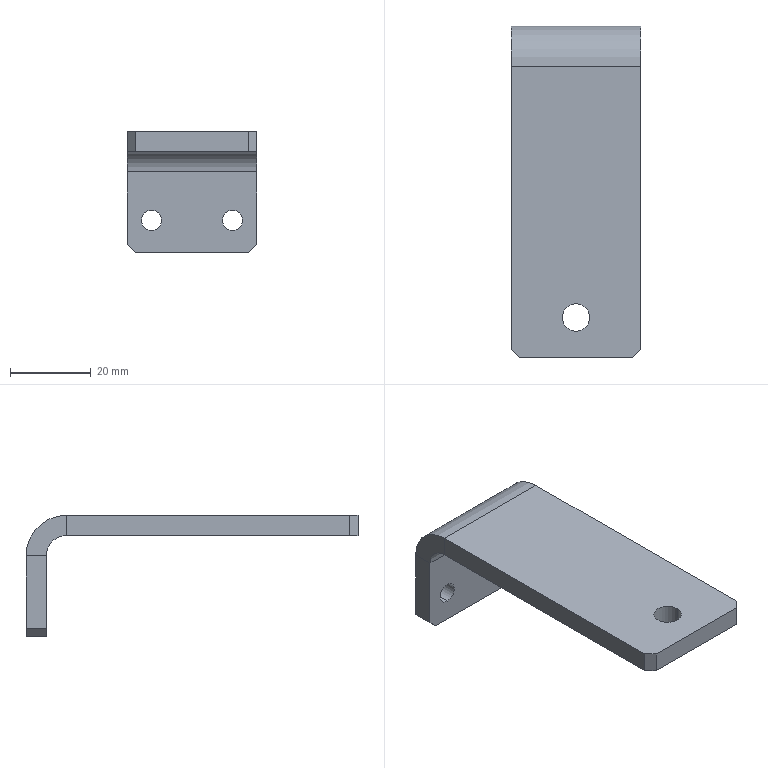Part | SolidWorks | features HoleWzd 2, Chamfer 1, EdgeFlange 1, FlatPattern 1, SMBaseFlange 1, SheetMetal 1 | 1 solid | 24 faces | box 32 x 82 x 30 mm | volume 16187 mm3 | plane 16 | cylinder 8 | commonest cylinder face diameters 5 x4 6.8 x2 10 x1 20 x1
STEP:
#1=CARTESIAN_POINT('',(-5.502,-25.632,-5.));
#2=VERTEX_POINT('',#1);
#3=CARTESIAN_POINT('',(1.298,-25.632,-5.));
#4=VERTEX_POINT('',#3);
#5=CARTESIAN_POINT('',(-2.102,-25.632,-5.));
#6=DIRECTION('',(0.,0.,1.));
#7=DIRECTION('',(1.,0.,0.));
#8=AXIS2_PLACEMENT_3D('',#5,#6,#7);
#9=CIRCLE('',#8,3.4);
#10=EDGE_CURVE('',#2,#4,#9,.T.);
#11=ORIENTED_EDGE('',*,*,#10,.F.);
#12=CARTESIAN_POINT('',(-5.502,-25.632,0.));
#13=VERTEX_POINT('',#12);
#14=CARTESIAN_POINT('',(-5.502,-25.632,0.));
#15=DIRECTION('',(0.,0.,1.));
#16=VECTOR('',#15,1000.);
#17=LINE('',#14,#16);
#18=EDGE_CURVE('',#2,#13,#17,.T.);
#19=ORIENTED_EDGE('',*,*,#18,.T.);
#20=CARTESIAN_POINT('',(1.298,-25.632,0.));
#21=VERTEX_POINT('',#20);
#22=CARTESIAN_POINT('',(-2.102,-25.632,0.));
#23=DIRECTION('',(0.,0.,1.));
#24=DIRECTION('',(1.,0.,0.));
#25=AXIS2_PLACEMENT_3D('',#22,#23,#24);
#26=CIRCLE('',#25,3.4);
#27=EDGE_CURVE('',#13,#21,#26,.T.);
#28=ORIENTED_EDGE('',*,*,#27,.T.);
#29=CARTESIAN_POINT('',(1.298,-25.632,0.));
#30=DIRECTION('',(0.,0.,1.));
#31=VECTOR('',#30,1000.);
#32=LINE('',#29,#31);
#33=EDGE_CURVE('',#4,#21,#32,.T.);
#34=ORIENTED_EDGE('',*,*,#33,.F.);
#35=EDGE_LOOP('',(#11,#19,#28,#34));
#36=FACE_OUTER_BOUND('',#35,.T.);
#37=CARTESIAN_POINT('',(-2.102,-25.632,0.));
#38=DIRECTION('',(0.,0.,1.));
#39=DIRECTION('',(1.,0.,0.));
#40=AXIS2_PLACEMENT_3D('',#37,#38,#39);
#41=CYLINDRICAL_SURFACE('',#40,3.4);
#42=ADVANCED_FACE('',(#36),#41,.F.);
#43=CARTESIAN_POINT('',(-12.102,41.368,-24.5));
#44=VERTEX_POINT('',#43);
#45=CARTESIAN_POINT('',(-12.102,41.368,-19.5));
#46=VERTEX_POINT('',#45);
#47=CARTESIAN_POINT('',(-12.102,41.368,-22.));
#48=DIRECTION('',(0.,1.,0.));
#49=DIRECTION('',(0.,0.,1.));
#50=AXIS2_PLACEMENT_3D('',#47,#48,#49);
#51=CIRCLE('',#50,2.5);
#52=EDGE_CURVE('',#44,#46,#51,.T.);
#53=ORIENTED_EDGE('',*,*,#52,.F.);
#54=CARTESIAN_POINT('',(-12.102,46.368,-24.5));
#55=VERTEX_POINT('',#54);
#56=CARTESIAN_POINT('',(-12.102,46.368,-24.5));
#57=DIRECTION('',(0.,1.,0.));
#58=VECTOR('',#57,1000.);
#59=LINE('',#56,#58);
#60=EDGE_CURVE('',#44,#55,#59,.T.);
#61=ORIENTED_EDGE('',*,*,#60,.T.);
#62=CARTESIAN_POINT('',(-12.102,46.368,-19.5));
#63=VERTEX_POINT('',#62);
#64=CARTESIAN_POINT('',(-12.102,46.368,-22.));
#65=DIRECTION('',(0.,1.,0.));
#66=DIRECTION('',(0.,0.,1.));
#67=AXIS2_PLACEMENT_3D('',#64,#65,#66);
#68=CIRCLE('',#67,2.5);
#69=EDGE_CURVE('',#55,#63,#68,.T.);
#70=ORIENTED_EDGE('',*,*,#69,.T.);
#71=CARTESIAN_POINT('',(-12.102,46.368,-19.5));
#72=DIRECTION('',(0.,1.,0.));
#73=VECTOR('',#72,1000.);
#74=LINE('',#71,#73);
#75=EDGE_CURVE('',#46,#63,#74,.T.);
#76=ORIENTED_EDGE('',*,*,#75,.F.);
#77=EDGE_LOOP('',(#53,#61,#70,#76));
#78=FACE_OUTER_BOUND('',#77,.T.);
#79=CARTESIAN_POINT('',(-12.102,46.368,-22.));
#80=DIRECTION('',(0.,1.,0.));
#81=DIRECTION('',(0.,0.,1.));
#82=AXIS2_PLACEMENT_3D('',#79,#80,#81);
#83=CYLINDRICAL_SURFACE('',#82,2.5);
#84=ADVANCED_FACE('',(#78),#83,.F.);
#85=CARTESIAN_POINT('',(7.898,41.368,-24.5));
#86=VERTEX_POINT('',#85);
#87=CARTESIAN_POINT('',(7.898,41.368,-19.5));
#88=VERTEX_POINT('',#87);
#89=CARTESIAN_POINT('',(7.898,41.368,-22.));
#90=DIRECTION('',(0.,1.,0.));
#91=DIRECTION('',(0.,0.,1.));
#92=AXIS2_PLACEMENT_3D('',#89,#90,#91);
#93=CIRCLE('',#92,2.5);
#94=EDGE_CURVE('',#86,#88,#93,.T.);
#95=ORIENTED_EDGE('',*,*,#94,.F.);
#96=CARTESIAN_POINT('',(7.898,46.368,-24.5));
#97=VERTEX_POINT('',#96);
#98=CARTESIAN_POINT('',(7.898,46.368,-24.5));
#99=DIRECTION('',(0.,1.,0.));
#100=VECTOR('',#99,1000.);
#101=LINE('',#98,#100);
#102=EDGE_CURVE('',#86,#97,#101,.T.);
#103=ORIENTED_EDGE('',*,*,#102,.T.);
#104=CARTESIAN_POINT('',(7.898,46.368,-19.5));
#105=VERTEX_POINT('',#104);
#106=CARTESIAN_POINT('',(7.898,46.368,-22.));
#107=DIRECTION('',(0.,1.,0.));
#108=DIRECTION('',(0.,0.,1.));
#109=AXIS2_PLACEMENT_3D('',#106,#107,#108);
#110=CIRCLE('',#109,2.5);
#111=EDGE_CURVE('',#97,#105,#110,.T.);
#112=ORIENTED_EDGE('',*,*,#111,.T.);
#113=CARTESIAN_POINT('',(7.898,46.368,-19.5));
#114=DIRECTION('',(0.,1.,0.));
#115=VECTOR('',#114,1000.);
#116=LINE('',#113,#115);
#117=EDGE_CURVE('',#88,#105,#116,.T.);
#118=ORIENTED_EDGE('',*,*,#117,.F.);
#119=EDGE_LOOP('',(#95,#103,#112,#118));
#120=FACE_OUTER_BOUND('',#119,.T.);
#121=CARTESIAN_POINT('',(7.898,46.368,-22.));
#122=DIRECTION('',(0.,1.,0.));
#123=DIRECTION('',(0.,0.,1.));
#124=AXIS2_PLACEMENT_3D('',#121,#122,#123);
#125=CYLINDRICAL_SURFACE('',#124,2.5);
#126=ADVANCED_FACE('',(#120),#125,.F.);
#127=CARTESIAN_POINT('',(13.898,-33.632,0.));
#128=VERTEX_POINT('',#127);
#129=CARTESIAN_POINT('',(13.898,36.368,0.));
#130=VERTEX_POINT('',#129);
#131=CARTESIAN_POINT('',(13.898,46.368,0.));
#132=DIRECTION('',(0.,1.,0.));
#133=VECTOR('',#132,1000.);
#134=LINE('',#131,#133);
#135=EDGE_CURVE('',#128,#130,#134,.T.);
#136=ORIENTED_EDGE('',*,*,#135,.F.);
#137=CARTESIAN_POINT('',(13.898,-33.632,-5.));
#138=VERTEX_POINT('',#137);
#139=CARTESIAN_POINT('',(13.898,-33.632,-5.));
#140=DIRECTION('',(0.,0.,-1.));
#141=VECTOR('',#140,1000.);
#142=LINE('',#139,#141);
#143=EDGE_CURVE('',#128,#138,#142,.T.);
#144=ORIENTED_EDGE('',*,*,#143,.T.);
#145=CARTESIAN_POINT('',(13.898,36.368,-5.));
#146=VERTEX_POINT('',#145);
#147=CARTESIAN_POINT('',(13.898,46.368,-5.));
#148=DIRECTION('',(0.,1.,0.));
#149=VECTOR('',#148,1000.);
#150=LINE('',#147,#149);
#151=EDGE_CURVE('',#138,#146,#150,.T.);
#152=ORIENTED_EDGE('',*,*,#151,.T.);
#153=CARTESIAN_POINT('',(13.898,36.368,-5.));
#154=DIRECTION('',(0.,0.,1.));
#155=VECTOR('',#154,1000.);
#156=LINE('',#153,#155);
#157=EDGE_CURVE('',#146,#130,#156,.T.);
#158=ORIENTED_EDGE('',*,*,#157,.T.);
#159=EDGE_LOOP('',(#136,#144,#152,#158));
#160=FACE_OUTER_BOUND('',#159,.T.);
#161=CARTESIAN_POINT('',(13.898,46.368,-5.));
#162=DIRECTION('',(1.,0.,0.));
#163=DIRECTION('',(0.,1.,0.));
#164=AXIS2_PLACEMENT_3D('',#161,#162,#163);
#165=PLANE('',#164);
#166=ADVANCED_FACE('',(#160),#165,.T.);
#167=CARTESIAN_POINT('',(-2.102,-25.632,-5.));
#168=DIRECTION('',(0.,0.,1.));
#169=DIRECTION('',(1.,0.,0.));
#170=AXIS2_PLACEMENT_3D('',#167,#168,#169);
#171=CIRCLE('',#170,3.4);
#172=EDGE_CURVE('',#4,#2,#171,.T.);
#173=ORIENTED_EDGE('',*,*,#172,.T.);
#174=ORIENTED_EDGE('',*,*,#10,.T.);
#175=EDGE_LOOP('',(#173,#174));
#176=FACE_BOUND('',#175,.T.);
#177=CARTESIAN_POINT('',(-16.102,-35.632,-5.));
#178=VERTEX_POINT('',#177);
#179=CARTESIAN_POINT('',(11.898,-35.632,-5.));
#180=VERTEX_POINT('',#179);
#181=CARTESIAN_POINT('',(-18.102,-35.632,-5.));
#182=DIRECTION('',(1.,0.,0.));
#183=VECTOR('',#182,1000.);
#184=LINE('',#181,#183);
#185=EDGE_CURVE('',#178,#180,#184,.T.);
#186=ORIENTED_EDGE('',*,*,#185,.F.);
#187=CARTESIAN_POINT('',(-18.102,-33.632,-5.));
#188=VERTEX_POINT('',#187);
#189=CARTESIAN_POINT('',(-18.102,-33.632,-5.));
#190=DIRECTION('',(-0.7071,0.7071,0.));
#191=VECTOR('',#190,1000.);
#192=LINE('',#189,#191);
#193=EDGE_CURVE('',#178,#188,#192,.T.);
#194=ORIENTED_EDGE('',*,*,#193,.T.);
#195=CARTESIAN_POINT('',(-18.102,36.368,-5.));
#196=VERTEX_POINT('',#195);
#197=CARTESIAN_POINT('',(-18.102,46.368,-5.));
#198=DIRECTION('',(0.,-1.,0.));
#199=VECTOR('',#198,1000.);
#200=LINE('',#197,#199);
#201=EDGE_CURVE('',#196,#188,#200,.T.);
#202=ORIENTED_EDGE('',*,*,#201,.F.);
#203=CARTESIAN_POINT('',(13.898,36.368,-5.));
#204=DIRECTION('',(-1.,0.,0.));
#205=VECTOR('',#204,1000.);
#206=LINE('',#203,#205);
#207=EDGE_CURVE('',#146,#196,#206,.T.);
#208=ORIENTED_EDGE('',*,*,#207,.F.);
#209=ORIENTED_EDGE('',*,*,#151,.F.);
#210=CARTESIAN_POINT('',(11.898,-35.632,-5.));
#211=DIRECTION('',(-0.7071,-0.7071,0.));
#212=VECTOR('',#211,1000.);
#213=LINE('',#210,#212);
#214=EDGE_CURVE('',#138,#180,#213,.T.);
#215=ORIENTED_EDGE('',*,*,#214,.T.);
#216=EDGE_LOOP('',(#186,#194,#202,#208,#209,#215));
#217=FACE_OUTER_BOUND('',#216,.T.);
#218=CARTESIAN_POINT('',(0.,0.,-5.));
#219=DIRECTION('',(0.,0.,1.));
#220=DIRECTION('',(1.,0.,0.));
#221=AXIS2_PLACEMENT_3D('',#218,#219,#220);
#222=PLANE('',#221);
#223=ADVANCED_FACE('',(#176,#217),#222,.F.);
#224=CARTESIAN_POINT('',(-2.102,-25.632,0.));
#225=DIRECTION('',(0.,0.,1.));
#226=DIRECTION('',(1.,0.,0.));
#227=AXIS2_PLACEMENT_3D('',#224,#225,#226);
#228=CIRCLE('',#227,3.4);
#229=EDGE_CURVE('',#21,#13,#228,.T.);
#230=ORIENTED_EDGE('',*,*,#229,.F.);
#231=ORIENTED_EDGE('',*,*,#27,.F.);
#232=EDGE_LOOP('',(#230,#231));
#233=FACE_BOUND('',#232,.T.);
#234=CARTESIAN_POINT('',(-18.102,36.368,0.));
#235=VERTEX_POINT('',#234);
#236=CARTESIAN_POINT('',(-18.102,-33.632,0.));
#237=VERTEX_POINT('',#236);
#238=CARTESIAN_POINT('',(-18.102,46.368,0.));
#239=DIRECTION('',(0.,-1.,0.));
#240=VECTOR('',#239,1000.);
#241=LINE('',#238,#240);
#242=EDGE_CURVE('',#235,#237,#241,.T.);
#243=ORIENTED_EDGE('',*,*,#242,.T.);
#244=CARTESIAN_POINT('',(-16.102,-35.632,0.));
#245=VERTEX_POINT('',#244);
#246=CARTESIAN_POINT('',(-25.867,-25.867,0.));
#247=DIRECTION('',(0.7071,-0.7071,0.));
#248=VECTOR('',#247,1000.);
#249=LINE('',#246,#248);
#250=EDGE_CURVE('',#237,#245,#249,.T.);
#251=ORIENTED_EDGE('',*,*,#250,.T.);
#252=CARTESIAN_POINT('',(11.898,-35.632,0.));
#253=VERTEX_POINT('',#252);
#254=CARTESIAN_POINT('',(-18.102,-35.632,0.));
#255=DIRECTION('',(1.,0.,0.));
#256=VECTOR('',#255,1000.);
#257=LINE('',#254,#256);
#258=EDGE_CURVE('',#245,#253,#257,.T.);
#259=ORIENTED_EDGE('',*,*,#258,.T.);
#260=CARTESIAN_POINT('',(23.765,-23.765,0.));
#261=DIRECTION('',(0.7071,0.7071,0.));
#262=VECTOR('',#261,1000.);
#263=LINE('',#260,#262);
#264=EDGE_CURVE('',#253,#128,#263,.T.);
#265=ORIENTED_EDGE('',*,*,#264,.T.);
#266=ORIENTED_EDGE('',*,*,#135,.T.);
#267=CARTESIAN_POINT('',(13.898,36.368,0.));
#268=DIRECTION('',(-1.,0.,0.));
#269=VECTOR('',#268,1000.);
#270=LINE('',#267,#269);
#271=EDGE_CURVE('',#130,#235,#270,.T.);
#272=ORIENTED_EDGE('',*,*,#271,.T.);
#273=EDGE_LOOP('',(#243,#251,#259,#265,#266,#272));
#274=FACE_OUTER_BOUND('',#273,.T.);
#275=CARTESIAN_POINT('',(0.,0.,0.));
#276=DIRECTION('',(0.,0.,1.));
#277=DIRECTION('',(1.,0.,0.));
#278=AXIS2_PLACEMENT_3D('',#275,#276,#277);
#279=PLANE('',#278);
#280=ADVANCED_FACE('',(#233,#274),#279,.T.);
#281=ORIENTED_EDGE('',*,*,#201,.T.);
#282=CARTESIAN_POINT('',(-18.102,-33.632,-5.));
#283=DIRECTION('',(0.,0.,1.));
#284=VECTOR('',#283,1000.);
#285=LINE('',#282,#284);
#286=EDGE_CURVE('',#188,#237,#285,.T.);
#287=ORIENTED_EDGE('',*,*,#286,.T.);
#288=ORIENTED_EDGE('',*,*,#242,.F.);
#289=CARTESIAN_POINT('',(-18.102,36.368,-5.));
#290=DIRECTION('',(0.,0.,1.));
#291=VECTOR('',#290,1000.);
#292=LINE('',#289,#291);
#293=EDGE_CURVE('',#196,#235,#292,.T.);
#294=ORIENTED_EDGE('',*,*,#293,.F.);
#295=EDGE_LOOP('',(#281,#287,#288,#294));
#296=FACE_OUTER_BOUND('',#295,.T.);
#297=CARTESIAN_POINT('',(-18.102,46.368,-5.));
#298=DIRECTION('',(-1.,0.,0.));
#299=DIRECTION('',(0.,-1.,0.));
#300=AXIS2_PLACEMENT_3D('',#297,#298,#299);
#301=PLANE('',#300);
#302=ADVANCED_FACE('',(#296),#301,.T.);
#303=ORIENTED_EDGE('',*,*,#258,.F.);
#304=CARTESIAN_POINT('',(-16.102,-35.632,-5.));
#305=DIRECTION('',(0.,0.,-1.));
#306=VECTOR('',#305,1000.);
#307=LINE('',#304,#306);
#308=EDGE_CURVE('',#245,#178,#307,.T.);
#309=ORIENTED_EDGE('',*,*,#308,.T.);
#310=ORIENTED_EDGE('',*,*,#185,.T.);
#311=CARTESIAN_POINT('',(11.898,-35.632,-5.));
#312=DIRECTION('',(0.,0.,1.));
#313=VECTOR('',#312,1000.);
#314=LINE('',#311,#313);
#315=EDGE_CURVE('',#180,#253,#314,.T.);
#316=ORIENTED_EDGE('',*,*,#315,.T.);
#317=EDGE_LOOP('',(#303,#309,#310,#316));
#318=FACE_OUTER_BOUND('',#317,.T.);
#319=CARTESIAN_POINT('',(-18.102,-35.632,-5.));
#320=DIRECTION('',(0.,-1.,0.));
#321=DIRECTION('',(0.,0.,-1.));
#322=AXIS2_PLACEMENT_3D('',#319,#320,#321);
#323=PLANE('',#322);
#324=ADVANCED_FACE('',(#318),#323,.T.);
#325=CARTESIAN_POINT('',(-18.102,41.368,-10.));
#326=VERTEX_POINT('',#325);
#327=CARTESIAN_POINT('',(-18.102,46.368,-10.));
#328=VERTEX_POINT('',#327);
#329=CARTESIAN_POINT('',(-18.102,46.368,-10.));
#330=DIRECTION('',(0.,1.,0.));
#331=VECTOR('',#330,1000.);
#332=LINE('',#329,#331);
#333=EDGE_CURVE('',#326,#328,#332,.T.);
#334=ORIENTED_EDGE('',*,*,#333,.F.);
#335=CARTESIAN_POINT('',(-18.102,36.368,-10.));
#336=DIRECTION('',(-1.,0.,0.));
#337=DIRECTION('',(0.,0.,-1.));
#338=AXIS2_PLACEMENT_3D('',#335,#336,#337);
#339=CIRCLE('',#338,5.);
#340=EDGE_CURVE('',#196,#326,#339,.T.);
#341=ORIENTED_EDGE('',*,*,#340,.F.);
#342=ORIENTED_EDGE('',*,*,#293,.T.);
#343=CARTESIAN_POINT('',(-18.102,36.368,-10.));
#344=DIRECTION('',(-1.,0.,0.));
#345=DIRECTION('',(0.,0.,-1.));
#346=AXIS2_PLACEMENT_3D('',#343,#344,#345);
#347=CIRCLE('',#346,10.);
#348=EDGE_CURVE('',#235,#328,#347,.T.);
#349=ORIENTED_EDGE('',*,*,#348,.T.);
#350=EDGE_LOOP('',(#334,#341,#342,#349));
#351=FACE_OUTER_BOUND('',#350,.T.);
#352=CARTESIAN_POINT('',(-18.102,36.368,-10.));
#353=DIRECTION('',(-1.,0.,0.));
#354=DIRECTION('',(0.,0.,1.));
#355=AXIS2_PLACEMENT_3D('',#352,#353,#354);
#356=PLANE('',#355);
#357=ADVANCED_FACE('',(#351),#356,.T.);
#358=CARTESIAN_POINT('',(13.898,41.368,-10.));
#359=VERTEX_POINT('',#358);
#360=CARTESIAN_POINT('',(13.898,36.368,-10.));
#361=DIRECTION('',(1.,0.,0.));
#362=DIRECTION('',(0.,0.,-1.));
#363=AXIS2_PLACEMENT_3D('',#360,#361,#362);
#364=CIRCLE('',#363,5.);
#365=EDGE_CURVE('',#359,#146,#364,.T.);
#366=ORIENTED_EDGE('',*,*,#365,.F.);
#367=CARTESIAN_POINT('',(13.898,46.368,-10.));
#368=VERTEX_POINT('',#367);
#369=CARTESIAN_POINT('',(13.898,41.368,-10.));
#370=DIRECTION('',(0.,1.,0.));
#371=VECTOR('',#370,1000.);
#372=LINE('',#369,#371);
#373=EDGE_CURVE('',#359,#368,#372,.T.);
#374=ORIENTED_EDGE('',*,*,#373,.T.);
#375=CARTESIAN_POINT('',(13.898,36.368,-10.));
#376=DIRECTION('',(1.,0.,0.));
#377=DIRECTION('',(0.,0.,-1.));
#378=AXIS2_PLACEMENT_3D('',#375,#376,#377);
#379=CIRCLE('',#378,10.);
#380=EDGE_CURVE('',#368,#130,#379,.T.);
#381=ORIENTED_EDGE('',*,*,#380,.T.);
#382=ORIENTED_EDGE('',*,*,#157,.F.);
#383=EDGE_LOOP('',(#366,#374,#381,#382));
#384=FACE_OUTER_BOUND('',#383,.T.);
#385=CARTESIAN_POINT('',(13.898,36.368,-10.));
#386=DIRECTION('',(-1.,0.,0.));
#387=DIRECTION('',(0.,0.,1.));
#388=AXIS2_PLACEMENT_3D('',#385,#386,#387);
#389=PLANE('',#388);
#390=ADVANCED_FACE('',(#384),#389,.F.);
#391=ORIENTED_EDGE('',*,*,#271,.F.);
#392=ORIENTED_EDGE('',*,*,#380,.F.);
#393=CARTESIAN_POINT('',(0.,46.368,-10.));
#394=DIRECTION('',(1.,0.,0.));
#395=VECTOR('',#394,1000.);
#396=LINE('',#393,#395);
#397=EDGE_CURVE('',#328,#368,#396,.T.);
#398=ORIENTED_EDGE('',*,*,#397,.F.);
#399=ORIENTED_EDGE('',*,*,#348,.F.);
#400=EDGE_LOOP('',(#391,#392,#398,#399));
#401=FACE_OUTER_BOUND('',#400,.T.);
#402=CARTESIAN_POINT('',(13.898,36.368,-10.));
#403=DIRECTION('',(1.,0.,0.));
#404=DIRECTION('',(0.,1.,0.));
#405=AXIS2_PLACEMENT_3D('',#402,#403,#404);
#406=CYLINDRICAL_SURFACE('',#405,10.);
#407=ADVANCED_FACE('',(#401),#406,.T.);
#408=ORIENTED_EDGE('',*,*,#207,.T.);
#409=ORIENTED_EDGE('',*,*,#340,.T.);
#410=CARTESIAN_POINT('',(-18.102,41.368,-10.));
#411=DIRECTION('',(1.,0.,0.));
#412=VECTOR('',#411,1000.);
#413=LINE('',#410,#412);
#414=EDGE_CURVE('',#326,#359,#413,.T.);
#415=ORIENTED_EDGE('',*,*,#414,.T.);
#416=ORIENTED_EDGE('',*,*,#365,.T.);
#417=EDGE_LOOP('',(#408,#409,#415,#416));
#418=FACE_OUTER_BOUND('',#417,.T.);
#419=CARTESIAN_POINT('',(13.898,36.368,-10.));
#420=DIRECTION('',(1.,0.,0.));
#421=DIRECTION('',(0.,1.,0.));
#422=AXIS2_PLACEMENT_3D('',#419,#420,#421);
#423=CYLINDRICAL_SURFACE('',#422,5.);
#424=ADVANCED_FACE('',(#418),#423,.F.);
#425=CARTESIAN_POINT('',(13.898,41.368,-28.));
#426=VERTEX_POINT('',#425);
#427=CARTESIAN_POINT('',(13.898,41.368,0.));
#428=DIRECTION('',(0.,0.,1.));
#429=VECTOR('',#428,1000.);
#430=LINE('',#427,#429);
#431=EDGE_CURVE('',#426,#359,#430,.T.);
#432=ORIENTED_EDGE('',*,*,#431,.F.);
#433=CARTESIAN_POINT('',(13.898,46.368,-28.));
#434=VERTEX_POINT('',#433);
#435=CARTESIAN_POINT('',(13.898,46.368,-28.));
#436=DIRECTION('',(0.,1.,0.));
#437=VECTOR('',#436,1000.);
#438=LINE('',#435,#437);
#439=EDGE_CURVE('',#426,#434,#438,.T.);
#440=ORIENTED_EDGE('',*,*,#439,.T.);
#441=CARTESIAN_POINT('',(13.898,46.368,-5.));
#442=DIRECTION('',(0.,0.,1.));
#443=VECTOR('',#442,1000.);
#444=LINE('',#441,#443);
#445=EDGE_CURVE('',#434,#368,#444,.T.);
#446=ORIENTED_EDGE('',*,*,#445,.T.);
#447=ORIENTED_EDGE('',*,*,#373,.F.);
#448=EDGE_LOOP('',(#432,#440,#446,#447));
#449=FACE_OUTER_BOUND('',#448,.T.);
#450=CARTESIAN_POINT('',(13.898,46.368,-5.));
#451=DIRECTION('',(1.,0.,0.));
#452=DIRECTION('',(0.,0.,-1.));
#453=AXIS2_PLACEMENT_3D('',#450,#451,#452);
#454=PLANE('',#453);
#455=ADVANCED_FACE('',(#449),#454,.T.);
#456=CARTESIAN_POINT('',(-18.102,46.368,-28.));
#457=VERTEX_POINT('',#456);
#458=CARTESIAN_POINT('',(-18.102,46.368,-30.));
#459=DIRECTION('',(0.,0.,-1.));
#460=VECTOR('',#459,1000.);
#461=LINE('',#458,#460);
#462=EDGE_CURVE('',#328,#457,#461,.T.);
#463=ORIENTED_EDGE('',*,*,#462,.T.);
#464=CARTESIAN_POINT('',(-18.102,41.368,-28.));
#465=VERTEX_POINT('',#464);
#466=CARTESIAN_POINT('',(-18.102,46.368,-28.));
#467=DIRECTION('',(0.,-1.,0.));
#468=VECTOR('',#467,1000.);
#469=LINE('',#466,#468);
#470=EDGE_CURVE('',#457,#465,#469,.T.);
#471=ORIENTED_EDGE('',*,*,#470,.T.);
#472=CARTESIAN_POINT('',(-18.102,41.368,0.));
#473=DIRECTION('',(0.,0.,-1.));
#474=VECTOR('',#473,1000.);
#475=LINE('',#472,#474);
#476=EDGE_CURVE('',#326,#465,#475,.T.);
#477=ORIENTED_EDGE('',*,*,#476,.F.);
#478=ORIENTED_EDGE('',*,*,#333,.T.);
#479=EDGE_LOOP('',(#463,#471,#477,#478));
#480=FACE_OUTER_BOUND('',#479,.T.);
#481=CARTESIAN_POINT('',(-18.102,46.368,-30.));
#482=DIRECTION('',(-1.,0.,0.));
#483=DIRECTION('',(0.,0.,1.));
#484=AXIS2_PLACEMENT_3D('',#481,#482,#483);
#485=PLANE('',#484);
#486=ADVANCED_FACE('',(#480),#485,.T.);
#487=CARTESIAN_POINT('',(-12.102,46.368,-22.));
#488=DIRECTION('',(0.,1.,0.));
#489=DIRECTION('',(0.,0.,1.));
#490=AXIS2_PLACEMENT_3D('',#487,#488,#489);
#491=CIRCLE('',#490,2.5);
#492=EDGE_CURVE('',#63,#55,#491,.T.);
#493=ORIENTED_EDGE('',*,*,#492,.F.);
#494=ORIENTED_EDGE('',*,*,#69,.F.);
#495=EDGE_LOOP('',(#493,#494));
#496=FACE_BOUND('',#495,.T.);
#497=CARTESIAN_POINT('',(7.898,46.368,-22.));
#498=DIRECTION('',(0.,1.,0.));
#499=DIRECTION('',(0.,0.,1.));
#500=AXIS2_PLACEMENT_3D('',#497,#498,#499);
#501=CIRCLE('',#500,2.5);
#502=EDGE_CURVE('',#105,#97,#501,.T.);
#503=ORIENTED_EDGE('',*,*,#502,.F.);
#504=ORIENTED_EDGE('',*,*,#111,.F.);
#505=EDGE_LOOP('',(#503,#504));
#506=FACE_BOUND('',#505,.T.);
#507=CARTESIAN_POINT('',(-16.102,46.368,-30.));
#508=VERTEX_POINT('',#507);
#509=CARTESIAN_POINT('',(11.898,46.368,-30.));
#510=VERTEX_POINT('',#509);
#511=CARTESIAN_POINT('',(13.898,46.368,-30.));
#512=DIRECTION('',(1.,0.,0.));
#513=VECTOR('',#512,1000.);
#514=LINE('',#511,#513);
#515=EDGE_CURVE('',#508,#510,#514,.T.);
#516=ORIENTED_EDGE('',*,*,#515,.F.);
#517=CARTESIAN_POINT('',(-23.051,46.368,-23.051));
#518=DIRECTION('',(-0.7071,0.,0.7071));
#519=VECTOR('',#518,1000.);
#520=LINE('',#517,#519);
#521=EDGE_CURVE('',#508,#457,#520,.T.);
#522=ORIENTED_EDGE('',*,*,#521,.T.);
#523=ORIENTED_EDGE('',*,*,#462,.F.);
#524=ORIENTED_EDGE('',*,*,#397,.T.);
#525=ORIENTED_EDGE('',*,*,#445,.F.);
#526=CARTESIAN_POINT('',(20.949,46.368,-20.949));
#527=DIRECTION('',(-0.7071,0.,-0.7071));
#528=VECTOR('',#527,1000.);
#529=LINE('',#526,#528);
#530=EDGE_CURVE('',#434,#510,#529,.T.);
#531=ORIENTED_EDGE('',*,*,#530,.T.);
#532=EDGE_LOOP('',(#516,#522,#523,#524,#525,#531));
#533=FACE_OUTER_BOUND('',#532,.T.);
#534=CARTESIAN_POINT('',(0.,46.368,0.));
#535=DIRECTION('',(0.,1.,0.));
#536=DIRECTION('',(0.,0.,1.));
#537=AXIS2_PLACEMENT_3D('',#534,#535,#536);
#538=PLANE('',#537);
#539=ADVANCED_FACE('',(#496,#506,#533),#538,.T.);
#540=CARTESIAN_POINT('',(-12.102,41.368,-22.));
#541=DIRECTION('',(0.,1.,0.));
#542=DIRECTION('',(0.,0.,1.));
#543=AXIS2_PLACEMENT_3D('',#540,#541,#542);
#544=CIRCLE('',#543,2.5);
#545=EDGE_CURVE('',#46,#44,#544,.T.);
#546=ORIENTED_EDGE('',*,*,#545,.T.);
#547=ORIENTED_EDGE('',*,*,#52,.T.);
#548=EDGE_LOOP('',(#546,#547));
#549=FACE_BOUND('',#548,.T.);
#550=CARTESIAN_POINT('',(7.898,41.368,-22.));
#551=DIRECTION('',(0.,1.,0.));
#552=DIRECTION('',(0.,0.,1.));
#553=AXIS2_PLACEMENT_3D('',#550,#551,#552);
#554=CIRCLE('',#553,2.5);
#555=EDGE_CURVE('',#88,#86,#554,.T.);
#556=ORIENTED_EDGE('',*,*,#555,.T.);
#557=ORIENTED_EDGE('',*,*,#94,.T.);
#558=EDGE_LOOP('',(#556,#557));
#559=FACE_BOUND('',#558,.T.);
#560=ORIENTED_EDGE('',*,*,#476,.T.);
#561=CARTESIAN_POINT('',(-16.102,41.368,-30.));
#562=VERTEX_POINT('',#561);
#563=CARTESIAN_POINT('',(-18.102,41.368,-28.));
#564=DIRECTION('',(0.7071,0.,-0.7071));
#565=VECTOR('',#564,1000.);
#566=LINE('',#563,#565);
#567=EDGE_CURVE('',#465,#562,#566,.T.);
#568=ORIENTED_EDGE('',*,*,#567,.T.);
#569=CARTESIAN_POINT('',(11.898,41.368,-30.));
#570=VERTEX_POINT('',#569);
#571=CARTESIAN_POINT('',(0.,41.368,-30.));
#572=DIRECTION('',(1.,0.,0.));
#573=VECTOR('',#572,1000.);
#574=LINE('',#571,#573);
#575=EDGE_CURVE('',#562,#570,#574,.T.);
#576=ORIENTED_EDGE('',*,*,#575,.T.);
#577=CARTESIAN_POINT('',(11.898,41.368,-30.));
#578=DIRECTION('',(0.7071,0.,0.7071));
#579=VECTOR('',#578,1000.);
#580=LINE('',#577,#579);
#581=EDGE_CURVE('',#570,#426,#580,.T.);
#582=ORIENTED_EDGE('',*,*,#581,.T.);
#583=ORIENTED_EDGE('',*,*,#431,.T.);
#584=ORIENTED_EDGE('',*,*,#414,.F.);
#585=EDGE_LOOP('',(#560,#568,#576,#582,#583,#584));
#586=FACE_OUTER_BOUND('',#585,.T.);
#587=CARTESIAN_POINT('',(0.,41.368,0.));
#588=DIRECTION('',(0.,1.,0.));
#589=DIRECTION('',(0.,0.,1.));
#590=AXIS2_PLACEMENT_3D('',#587,#588,#589);
#591=PLANE('',#590);
#592=ADVANCED_FACE('',(#549,#559,#586),#591,.F.);
#593=ORIENTED_EDGE('',*,*,#575,.F.);
#594=CARTESIAN_POINT('',(-16.102,46.368,-30.));
#595=DIRECTION('',(0.,1.,0.));
#596=VECTOR('',#595,1000.);
#597=LINE('',#594,#596);
#598=EDGE_CURVE('',#562,#508,#597,.T.);
#599=ORIENTED_EDGE('',*,*,#598,.T.);
#600=ORIENTED_EDGE('',*,*,#515,.T.);
#601=CARTESIAN_POINT('',(11.898,46.368,-30.));
#602=DIRECTION('',(0.,-1.,0.));
#603=VECTOR('',#602,1000.);
#604=LINE('',#601,#603);
#605=EDGE_CURVE('',#510,#570,#604,.T.);
#606=ORIENTED_EDGE('',*,*,#605,.T.);
#607=EDGE_LOOP('',(#593,#599,#600,#606));
#608=FACE_OUTER_BOUND('',#607,.T.);
#609=CARTESIAN_POINT('',(13.898,46.368,-30.));
#610=DIRECTION('',(0.,0.,-1.));
#611=DIRECTION('',(0.,1.,0.));
#612=AXIS2_PLACEMENT_3D('',#609,#610,#611);
#613=PLANE('',#612);
#614=ADVANCED_FACE('',(#608),#613,.T.);
#615=ORIENTED_EDGE('',*,*,#193,.F.);
#616=ORIENTED_EDGE('',*,*,#308,.F.);
#617=ORIENTED_EDGE('',*,*,#250,.F.);
#618=ORIENTED_EDGE('',*,*,#286,.F.);
#619=EDGE_LOOP('',(#615,#616,#617,#618));
#620=FACE_OUTER_BOUND('',#619,.T.);
#621=CARTESIAN_POINT('',(-18.102,-33.632,-5.));
#622=DIRECTION('',(0.7071,0.7071,0.));
#623=DIRECTION('',(0.,0.,1.));
#624=AXIS2_PLACEMENT_3D('',#621,#622,#623);
#625=PLANE('',#624);
#626=ADVANCED_FACE('',(#620),#625,.F.);
#627=ORIENTED_EDGE('',*,*,#214,.F.);
#628=ORIENTED_EDGE('',*,*,#143,.F.);
#629=ORIENTED_EDGE('',*,*,#264,.F.);
#630=ORIENTED_EDGE('',*,*,#315,.F.);
#631=EDGE_LOOP('',(#627,#628,#629,#630));
#632=FACE_OUTER_BOUND('',#631,.T.);
#633=CARTESIAN_POINT('',(11.898,-35.632,-5.));
#634=DIRECTION('',(-0.7071,0.7071,0.));
#635=DIRECTION('',(0.,0.,1.));
#636=AXIS2_PLACEMENT_3D('',#633,#634,#635);
#637=PLANE('',#636);
#638=ADVANCED_FACE('',(#632),#637,.F.);
#639=ORIENTED_EDGE('',*,*,#521,.F.);
#640=ORIENTED_EDGE('',*,*,#598,.F.);
#641=ORIENTED_EDGE('',*,*,#567,.F.);
#642=ORIENTED_EDGE('',*,*,#470,.F.);
#643=EDGE_LOOP('',(#639,#640,#641,#642));
#644=FACE_OUTER_BOUND('',#643,.T.);
#645=CARTESIAN_POINT('',(-18.102,46.368,-28.));
#646=DIRECTION('',(0.7071,0.,0.7071));
#647=DIRECTION('',(0.,-1.,0.));
#648=AXIS2_PLACEMENT_3D('',#645,#646,#647);
#649=PLANE('',#648);
#650=ADVANCED_FACE('',(#644),#649,.F.);
#651=ORIENTED_EDGE('',*,*,#530,.F.);
#652=ORIENTED_EDGE('',*,*,#439,.F.);
#653=ORIENTED_EDGE('',*,*,#581,.F.);
#654=ORIENTED_EDGE('',*,*,#605,.F.);
#655=EDGE_LOOP('',(#651,#652,#653,#654));
#656=FACE_OUTER_BOUND('',#655,.T.);
#657=CARTESIAN_POINT('',(11.898,46.368,-30.));
#658=DIRECTION('',(-0.7071,0.,0.7071));
#659=DIRECTION('',(0.,-1.,0.));
#660=AXIS2_PLACEMENT_3D('',#657,#658,#659);
#661=PLANE('',#660);
#662=ADVANCED_FACE('',(#656),#661,.F.);
#663=ORIENTED_EDGE('',*,*,#102,.F.);
#664=ORIENTED_EDGE('',*,*,#555,.F.);
#665=ORIENTED_EDGE('',*,*,#117,.T.);
#666=ORIENTED_EDGE('',*,*,#502,.T.);
#667=EDGE_LOOP('',(#663,#664,#665,#666));
#668=FACE_OUTER_BOUND('',#667,.T.);
#669=CARTESIAN_POINT('',(7.898,46.368,-22.));
#670=DIRECTION('',(0.,1.,0.));
#671=DIRECTION('',(0.,0.,1.));
#672=AXIS2_PLACEMENT_3D('',#669,#670,#671);
#673=CYLINDRICAL_SURFACE('',#672,2.5);
#674=ADVANCED_FACE('',(#668),#673,.F.);
#675=ORIENTED_EDGE('',*,*,#60,.F.);
#676=ORIENTED_EDGE('',*,*,#545,.F.);
#677=ORIENTED_EDGE('',*,*,#75,.T.);
#678=ORIENTED_EDGE('',*,*,#492,.T.);
#679=EDGE_LOOP('',(#675,#676,#677,#678));
#680=FACE_OUTER_BOUND('',#679,.T.);
#681=CARTESIAN_POINT('',(-12.102,46.368,-22.));
#682=DIRECTION('',(0.,1.,0.));
#683=DIRECTION('',(0.,0.,1.));
#684=AXIS2_PLACEMENT_3D('',#681,#682,#683);
#685=CYLINDRICAL_SURFACE('',#684,2.5);
#686=ADVANCED_FACE('',(#680),#685,.F.);
#687=ORIENTED_EDGE('',*,*,#18,.F.);
#688=ORIENTED_EDGE('',*,*,#172,.F.);
#689=ORIENTED_EDGE('',*,*,#33,.T.);
#690=ORIENTED_EDGE('',*,*,#229,.T.);
#691=EDGE_LOOP('',(#687,#688,#689,#690));
#692=FACE_OUTER_BOUND('',#691,.T.);
#693=CARTESIAN_POINT('',(-2.102,-25.632,0.));
#694=DIRECTION('',(0.,0.,1.));
#695=DIRECTION('',(1.,0.,0.));
#696=AXIS2_PLACEMENT_3D('',#693,#694,#695);
#697=CYLINDRICAL_SURFACE('',#696,3.4);
#698=ADVANCED_FACE('',(#692),#697,.F.);
#699=CLOSED_SHELL('',(#42,#84,#126,#166,#223,#280,#302,#324,#357,#390,#407,#424,#455,#486,#539,#592,#614,#626,#638,#650,#662,#674,#686,#698));
#700=MANIFOLD_SOLID_BREP('',#699);
#701=CARTESIAN_POINT('',(0.,0.,0.));
#702=DIRECTION('',(0.,0.,1.));
#703=DIRECTION('',(1.,0.,0.));
#704=AXIS2_PLACEMENT_3D('',#701,#702,#703);
#705=(LENGTH_UNIT()NAMED_UNIT(*)SI_UNIT(.MILLI.,.METRE.));
#706=UNCERTAINTY_MEASURE_WITH_UNIT(LENGTH_MEASURE(0.00001),#705,'','');
#707=(NAMED_UNIT(*)PLANE_ANGLE_UNIT()SI_UNIT($,.RADIAN.));
#708=(NAMED_UNIT(*)SI_UNIT($,.STERADIAN.)SOLID_ANGLE_UNIT());
#709=(GEOMETRIC_REPRESENTATION_CONTEXT(3)GLOBAL_UNCERTAINTY_ASSIGNED_CONTEXT((#706))GLOBAL_UNIT_ASSIGNED_CONTEXT((#705,#707,#708))REPRESENTATION_CONTEXT('',''));
#710=ADVANCED_BREP_SHAPE_REPRESENTATION('',(#700,#704),#709);